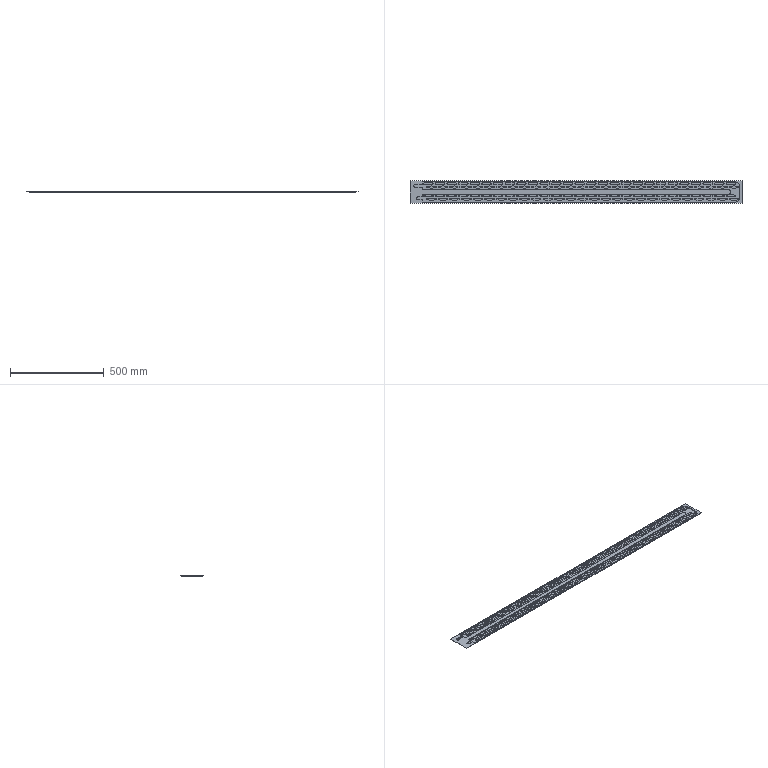Part | SolidWorks | features ICE 7, LPattern 2, BaseBody 1 | 1 solid | 2208 faces | box 1768 x 120 x 5 mm | volume 286159 mm3 | plane 1116 | cylinder 1092 | commonest cylinder face diameters 4 x324 6 x324 12 x218 10 x216 14 x2 18 x2